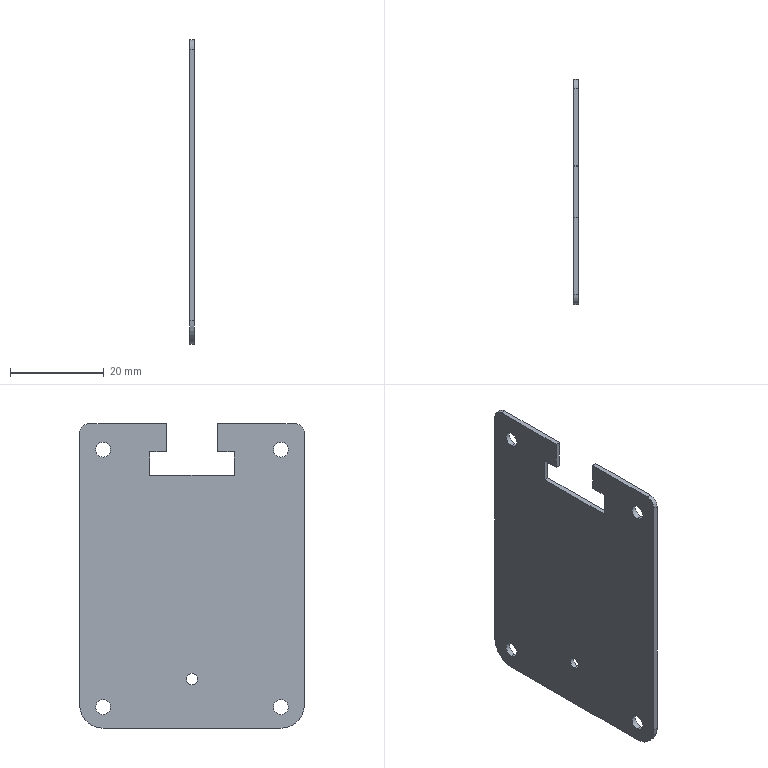Part | SolidWorks | features ICE 8, Fillet 2, Chamfer 1, Extrusion 1, HoleWzd 1 | 1 solid | 28 faces | box 1 x 48 x 65 mm | volume 2915 mm3 | cylinder 14 | plane 14 | commonest cylinder face diameters 3.2 x8 2.4 x2 4 x2 10 x2
STEP:
#1=CARTESIAN_POINT('',(20.,-19.,-26.4));
#2=VERTEX_POINT('',#1);
#3=CARTESIAN_POINT('',(20.,-19.,-29.6));
#4=VERTEX_POINT('',#3);
#5=CARTESIAN_POINT('',(20.,-19.,-28.));
#6=DIRECTION('',(1.,0.,0.));
#7=DIRECTION('',(0.,0.,-1.));
#8=AXIS2_PLACEMENT_3D('',#5,#6,#7);
#9=CIRCLE('',#8,1.6);
#10=EDGE_CURVE('',#2,#4,#9,.T.);
#11=ORIENTED_EDGE('',*,*,#10,.T.);
#12=CARTESIAN_POINT('',(19.,-19.,-29.6));
#13=VERTEX_POINT('',#12);
#14=CARTESIAN_POINT('',(139.,-19.,-29.6));
#15=DIRECTION('',(-1.,0.,0.));
#16=VECTOR('',#15,1000.);
#17=LINE('',#14,#16);
#18=EDGE_CURVE('',#4,#13,#17,.T.);
#19=ORIENTED_EDGE('',*,*,#18,.T.);
#20=CARTESIAN_POINT('',(19.,-19.,-26.4));
#21=VERTEX_POINT('',#20);
#22=CARTESIAN_POINT('',(19.,-19.,-28.));
#23=DIRECTION('',(-1.,0.,0.));
#24=DIRECTION('',(0.,0.,1.));
#25=AXIS2_PLACEMENT_3D('',#22,#23,#24);
#26=CIRCLE('',#25,1.6);
#27=EDGE_CURVE('',#13,#21,#26,.T.);
#28=ORIENTED_EDGE('',*,*,#27,.T.);
#29=CARTESIAN_POINT('',(139.,-19.,-26.4));
#30=DIRECTION('',(-1.,0.,0.));
#31=VECTOR('',#30,1000.);
#32=LINE('',#29,#31);
#33=EDGE_CURVE('',#2,#21,#32,.T.);
#34=ORIENTED_EDGE('',*,*,#33,.F.);
#35=EDGE_LOOP('',(#11,#19,#28,#34));
#36=FACE_OUTER_BOUND('',#35,.T.);
#37=CARTESIAN_POINT('',(139.,-19.,-28.));
#38=DIRECTION('',(-1.,0.,0.));
#39=DIRECTION('',(0.,0.,1.));
#40=AXIS2_PLACEMENT_3D('',#37,#38,#39);
#41=CYLINDRICAL_SURFACE('',#40,1.6);
#42=ADVANCED_FACE('',(#36),#41,.F.);
#43=CARTESIAN_POINT('',(20.,-19.,28.6));
#44=VERTEX_POINT('',#43);
#45=CARTESIAN_POINT('',(20.,-19.,25.4));
#46=VERTEX_POINT('',#45);
#47=CARTESIAN_POINT('',(20.,-19.,27.));
#48=DIRECTION('',(1.,0.,0.));
#49=DIRECTION('',(0.,0.,-1.));
#50=AXIS2_PLACEMENT_3D('',#47,#48,#49);
#51=CIRCLE('',#50,1.6);
#52=EDGE_CURVE('',#44,#46,#51,.T.);
#53=ORIENTED_EDGE('',*,*,#52,.T.);
#54=CARTESIAN_POINT('',(19.,-19.,25.4));
#55=VERTEX_POINT('',#54);
#56=CARTESIAN_POINT('',(139.,-19.,25.4));
#57=DIRECTION('',(-1.,0.,0.));
#58=VECTOR('',#57,1000.);
#59=LINE('',#56,#58);
#60=EDGE_CURVE('',#46,#55,#59,.T.);
#61=ORIENTED_EDGE('',*,*,#60,.T.);
#62=CARTESIAN_POINT('',(19.,-19.,28.6));
#63=VERTEX_POINT('',#62);
#64=CARTESIAN_POINT('',(19.,-19.,27.));
#65=DIRECTION('',(-1.,0.,0.));
#66=DIRECTION('',(0.,0.,1.));
#67=AXIS2_PLACEMENT_3D('',#64,#65,#66);
#68=CIRCLE('',#67,1.6);
#69=EDGE_CURVE('',#55,#63,#68,.T.);
#70=ORIENTED_EDGE('',*,*,#69,.T.);
#71=CARTESIAN_POINT('',(139.,-19.,28.6));
#72=DIRECTION('',(-1.,0.,0.));
#73=VECTOR('',#72,1000.);
#74=LINE('',#71,#73);
#75=EDGE_CURVE('',#44,#63,#74,.T.);
#76=ORIENTED_EDGE('',*,*,#75,.F.);
#77=EDGE_LOOP('',(#53,#61,#70,#76));
#78=FACE_OUTER_BOUND('',#77,.T.);
#79=CARTESIAN_POINT('',(139.,-19.,27.));
#80=DIRECTION('',(-1.,0.,0.));
#81=DIRECTION('',(0.,0.,1.));
#82=AXIS2_PLACEMENT_3D('',#79,#80,#81);
#83=CYLINDRICAL_SURFACE('',#82,1.6);
#84=ADVANCED_FACE('',(#78),#83,.F.);
#85=CARTESIAN_POINT('',(20.,19.,28.6));
#86=VERTEX_POINT('',#85);
#87=CARTESIAN_POINT('',(20.,19.,25.4));
#88=VERTEX_POINT('',#87);
#89=CARTESIAN_POINT('',(20.,19.,27.));
#90=DIRECTION('',(1.,0.,0.));
#91=DIRECTION('',(0.,0.,-1.));
#92=AXIS2_PLACEMENT_3D('',#89,#90,#91);
#93=CIRCLE('',#92,1.6);
#94=EDGE_CURVE('',#86,#88,#93,.T.);
#95=ORIENTED_EDGE('',*,*,#94,.T.);
#96=CARTESIAN_POINT('',(19.,19.,25.4));
#97=VERTEX_POINT('',#96);
#98=CARTESIAN_POINT('',(139.,19.,25.4));
#99=DIRECTION('',(-1.,0.,0.));
#100=VECTOR('',#99,1000.);
#101=LINE('',#98,#100);
#102=EDGE_CURVE('',#88,#97,#101,.T.);
#103=ORIENTED_EDGE('',*,*,#102,.T.);
#104=CARTESIAN_POINT('',(19.,19.,28.6));
#105=VERTEX_POINT('',#104);
#106=CARTESIAN_POINT('',(19.,19.,27.));
#107=DIRECTION('',(-1.,0.,0.));
#108=DIRECTION('',(0.,0.,-1.));
#109=AXIS2_PLACEMENT_3D('',#106,#107,#108);
#110=CIRCLE('',#109,1.6);
#111=EDGE_CURVE('',#97,#105,#110,.T.);
#112=ORIENTED_EDGE('',*,*,#111,.T.);
#113=CARTESIAN_POINT('',(139.,19.,28.6));
#114=DIRECTION('',(-1.,0.,0.));
#115=VECTOR('',#114,1000.);
#116=LINE('',#113,#115);
#117=EDGE_CURVE('',#86,#105,#116,.T.);
#118=ORIENTED_EDGE('',*,*,#117,.F.);
#119=EDGE_LOOP('',(#95,#103,#112,#118));
#120=FACE_OUTER_BOUND('',#119,.T.);
#121=CARTESIAN_POINT('',(139.,19.,27.));
#122=DIRECTION('',(-1.,0.,0.));
#123=DIRECTION('',(0.,0.,1.));
#124=AXIS2_PLACEMENT_3D('',#121,#122,#123);
#125=CYLINDRICAL_SURFACE('',#124,1.6);
#126=ADVANCED_FACE('',(#120),#125,.F.);
#127=CARTESIAN_POINT('',(20.,19.,-26.4));
#128=VERTEX_POINT('',#127);
#129=CARTESIAN_POINT('',(20.,19.,-29.6));
#130=VERTEX_POINT('',#129);
#131=CARTESIAN_POINT('',(20.,19.,-28.));
#132=DIRECTION('',(1.,0.,0.));
#133=DIRECTION('',(0.,0.,-1.));
#134=AXIS2_PLACEMENT_3D('',#131,#132,#133);
#135=CIRCLE('',#134,1.6);
#136=EDGE_CURVE('',#128,#130,#135,.T.);
#137=ORIENTED_EDGE('',*,*,#136,.T.);
#138=CARTESIAN_POINT('',(19.,19.,-29.6));
#139=VERTEX_POINT('',#138);
#140=CARTESIAN_POINT('',(139.,19.,-29.6));
#141=DIRECTION('',(-1.,0.,0.));
#142=VECTOR('',#141,1000.);
#143=LINE('',#140,#142);
#144=EDGE_CURVE('',#130,#139,#143,.T.);
#145=ORIENTED_EDGE('',*,*,#144,.T.);
#146=CARTESIAN_POINT('',(19.,19.,-26.4));
#147=VERTEX_POINT('',#146);
#148=CARTESIAN_POINT('',(19.,19.,-28.));
#149=DIRECTION('',(-1.,0.,0.));
#150=DIRECTION('',(0.,0.,1.));
#151=AXIS2_PLACEMENT_3D('',#148,#149,#150);
#152=CIRCLE('',#151,1.6);
#153=EDGE_CURVE('',#139,#147,#152,.T.);
#154=ORIENTED_EDGE('',*,*,#153,.T.);
#155=CARTESIAN_POINT('',(139.,19.,-26.4));
#156=DIRECTION('',(-1.,0.,0.));
#157=VECTOR('',#156,1000.);
#158=LINE('',#155,#157);
#159=EDGE_CURVE('',#128,#147,#158,.T.);
#160=ORIENTED_EDGE('',*,*,#159,.F.);
#161=EDGE_LOOP('',(#137,#145,#154,#160));
#162=FACE_OUTER_BOUND('',#161,.T.);
#163=CARTESIAN_POINT('',(139.,19.,-28.));
#164=DIRECTION('',(-1.,0.,0.));
#165=DIRECTION('',(0.,0.,1.));
#166=AXIS2_PLACEMENT_3D('',#163,#164,#165);
#167=CYLINDRICAL_SURFACE('',#166,1.6);
#168=ADVANCED_FACE('',(#162),#167,.F.);
#169=CARTESIAN_POINT('',(19.,0.,-23.2));
#170=VERTEX_POINT('',#169);
#171=CARTESIAN_POINT('',(19.,0.,-20.8));
#172=VERTEX_POINT('',#171);
#173=CARTESIAN_POINT('',(19.,0.,-22.));
#174=DIRECTION('',(-1.,0.,0.));
#175=DIRECTION('',(0.,0.,-1.));
#176=AXIS2_PLACEMENT_3D('',#173,#174,#175);
#177=CIRCLE('',#176,1.2);
#178=EDGE_CURVE('',#170,#172,#177,.T.);
#179=ORIENTED_EDGE('',*,*,#178,.T.);
#180=CARTESIAN_POINT('',(20.,0.,-20.8));
#181=VERTEX_POINT('',#180);
#182=CARTESIAN_POINT('',(14.,0.,-20.8));
#183=DIRECTION('',(1.,0.,0.));
#184=VECTOR('',#183,1000.);
#185=LINE('',#182,#184);
#186=EDGE_CURVE('',#172,#181,#185,.T.);
#187=ORIENTED_EDGE('',*,*,#186,.T.);
#188=CARTESIAN_POINT('',(20.,0.,-23.2));
#189=VERTEX_POINT('',#188);
#190=CARTESIAN_POINT('',(20.,0.,-22.));
#191=DIRECTION('',(1.,0.,0.));
#192=DIRECTION('',(0.,0.,-1.));
#193=AXIS2_PLACEMENT_3D('',#190,#191,#192);
#194=CIRCLE('',#193,1.2);
#195=EDGE_CURVE('',#181,#189,#194,.T.);
#196=ORIENTED_EDGE('',*,*,#195,.T.);
#197=CARTESIAN_POINT('',(14.,0.,-23.2));
#198=DIRECTION('',(1.,0.,0.));
#199=VECTOR('',#198,1000.);
#200=LINE('',#197,#199);
#201=EDGE_CURVE('',#170,#189,#200,.T.);
#202=ORIENTED_EDGE('',*,*,#201,.F.);
#203=EDGE_LOOP('',(#179,#187,#196,#202));
#204=FACE_OUTER_BOUND('',#203,.T.);
#205=CARTESIAN_POINT('',(14.,0.,-22.));
#206=DIRECTION('',(1.,0.,0.));
#207=DIRECTION('',(0.,0.,-1.));
#208=AXIS2_PLACEMENT_3D('',#205,#206,#207);
#209=CYLINDRICAL_SURFACE('',#208,1.2);
#210=ADVANCED_FACE('',(#204),#209,.F.);
#211=CARTESIAN_POINT('',(20.,22.,32.5));
#212=VERTEX_POINT('',#211);
#213=CARTESIAN_POINT('',(20.,5.5,32.5));
#214=VERTEX_POINT('',#213);
#215=CARTESIAN_POINT('',(20.,24.,32.5));
#216=DIRECTION('',(0.,-1.,0.));
#217=VECTOR('',#216,1000.);
#218=LINE('',#215,#217);
#219=EDGE_CURVE('',#212,#214,#218,.T.);
#220=ORIENTED_EDGE('',*,*,#219,.F.);
#221=CARTESIAN_POINT('',(19.,22.,32.5));
#222=VERTEX_POINT('',#221);
#223=CARTESIAN_POINT('',(20.,22.,32.5));
#224=DIRECTION('',(-1.,0.,0.));
#225=VECTOR('',#224,1000.);
#226=LINE('',#223,#225);
#227=EDGE_CURVE('',#212,#222,#226,.T.);
#228=ORIENTED_EDGE('',*,*,#227,.T.);
#229=CARTESIAN_POINT('',(19.,5.5,32.5));
#230=VERTEX_POINT('',#229);
#231=CARTESIAN_POINT('',(19.,24.,32.5));
#232=DIRECTION('',(0.,-1.,0.));
#233=VECTOR('',#232,1000.);
#234=LINE('',#231,#233);
#235=EDGE_CURVE('',#222,#230,#234,.T.);
#236=ORIENTED_EDGE('',*,*,#235,.T.);
#237=CARTESIAN_POINT('',(-60.,5.5,32.5));
#238=DIRECTION('',(1.,0.,0.));
#239=VECTOR('',#238,1000.);
#240=LINE('',#237,#239);
#241=EDGE_CURVE('',#230,#214,#240,.T.);
#242=ORIENTED_EDGE('',*,*,#241,.T.);
#243=EDGE_LOOP('',(#220,#228,#236,#242));
#244=FACE_OUTER_BOUND('',#243,.T.);
#245=CARTESIAN_POINT('',(20.,24.,32.5));
#246=DIRECTION('',(0.,0.,-1.));
#247=DIRECTION('',(0.,1.,0.));
#248=AXIS2_PLACEMENT_3D('',#245,#246,#247);
#249=PLANE('',#248);
#250=ADVANCED_FACE('',(#244),#249,.F.);
#251=CARTESIAN_POINT('',(20.,-19.,-32.5));
#252=VERTEX_POINT('',#251);
#253=CARTESIAN_POINT('',(19.,-19.,-32.5));
#254=VERTEX_POINT('',#253);
#255=CARTESIAN_POINT('',(20.,-19.,-32.5));
#256=DIRECTION('',(-1.,0.,0.));
#257=VECTOR('',#256,1000.);
#258=LINE('',#255,#257);
#259=EDGE_CURVE('',#252,#254,#258,.T.);
#260=ORIENTED_EDGE('',*,*,#259,.T.);
#261=CARTESIAN_POINT('',(19.,19.,-32.5));
#262=VERTEX_POINT('',#261);
#263=CARTESIAN_POINT('',(19.,24.,-32.5));
#264=DIRECTION('',(0.,1.,0.));
#265=VECTOR('',#264,1000.);
#266=LINE('',#263,#265);
#267=EDGE_CURVE('',#254,#262,#266,.T.);
#268=ORIENTED_EDGE('',*,*,#267,.T.);
#269=CARTESIAN_POINT('',(20.,19.,-32.5));
#270=VERTEX_POINT('',#269);
#271=CARTESIAN_POINT('',(20.,19.,-32.5));
#272=DIRECTION('',(1.,0.,0.));
#273=VECTOR('',#272,1000.);
#274=LINE('',#271,#273);
#275=EDGE_CURVE('',#262,#270,#274,.T.);
#276=ORIENTED_EDGE('',*,*,#275,.T.);
#277=CARTESIAN_POINT('',(20.,24.,-32.5));
#278=DIRECTION('',(0.,1.,0.));
#279=VECTOR('',#278,1000.);
#280=LINE('',#277,#279);
#281=EDGE_CURVE('',#252,#270,#280,.T.);
#282=ORIENTED_EDGE('',*,*,#281,.F.);
#283=EDGE_LOOP('',(#260,#268,#276,#282));
#284=FACE_OUTER_BOUND('',#283,.T.);
#285=CARTESIAN_POINT('',(20.,24.,-32.5));
#286=DIRECTION('',(0.,0.,1.));
#287=DIRECTION('',(0.,-1.,0.));
#288=AXIS2_PLACEMENT_3D('',#285,#286,#287);
#289=PLANE('',#288);
#290=ADVANCED_FACE('',(#284),#289,.F.);
#291=CARTESIAN_POINT('',(19.,24.,30.5));
#292=VERTEX_POINT('',#291);
#293=CARTESIAN_POINT('',(19.,24.,-27.5));
#294=VERTEX_POINT('',#293);
#295=CARTESIAN_POINT('',(19.,24.,-41.997));
#296=DIRECTION('',(0.,0.,-1.));
#297=VECTOR('',#296,1000.);
#298=LINE('',#295,#297);
#299=EDGE_CURVE('',#292,#294,#298,.T.);
#300=ORIENTED_EDGE('',*,*,#299,.F.);
#301=CARTESIAN_POINT('',(20.,24.,30.5));
#302=VERTEX_POINT('',#301);
#303=CARTESIAN_POINT('',(20.,24.,30.5));
#304=DIRECTION('',(1.,0.,0.));
#305=VECTOR('',#304,1000.);
#306=LINE('',#303,#305);
#307=EDGE_CURVE('',#292,#302,#306,.T.);
#308=ORIENTED_EDGE('',*,*,#307,.T.);
#309=CARTESIAN_POINT('',(20.,24.,-27.5));
#310=VERTEX_POINT('',#309);
#311=CARTESIAN_POINT('',(20.,24.,32.5));
#312=DIRECTION('',(0.,0.,1.));
#313=VECTOR('',#312,1000.);
#314=LINE('',#311,#313);
#315=EDGE_CURVE('',#310,#302,#314,.T.);
#316=ORIENTED_EDGE('',*,*,#315,.F.);
#317=CARTESIAN_POINT('',(20.,24.,-27.5));
#318=DIRECTION('',(-1.,0.,0.));
#319=VECTOR('',#318,1000.);
#320=LINE('',#317,#319);
#321=EDGE_CURVE('',#310,#294,#320,.T.);
#322=ORIENTED_EDGE('',*,*,#321,.T.);
#323=EDGE_LOOP('',(#300,#308,#316,#322));
#324=FACE_OUTER_BOUND('',#323,.T.);
#325=CARTESIAN_POINT('',(20.,24.,32.5));
#326=DIRECTION('',(0.,-1.,0.));
#327=DIRECTION('',(0.,0.,-1.));
#328=AXIS2_PLACEMENT_3D('',#325,#326,#327);
#329=PLANE('',#328);
#330=ADVANCED_FACE('',(#324),#329,.F.);
#331=CARTESIAN_POINT('',(19.,-5.5,32.5));
#332=VERTEX_POINT('',#331);
#333=CARTESIAN_POINT('',(19.,-22.,32.5));
#334=VERTEX_POINT('',#333);
#335=CARTESIAN_POINT('',(19.,24.,32.5));
#336=DIRECTION('',(0.,-1.,0.));
#337=VECTOR('',#336,1000.);
#338=LINE('',#335,#337);
#339=EDGE_CURVE('',#332,#334,#338,.T.);
#340=ORIENTED_EDGE('',*,*,#339,.T.);
#341=CARTESIAN_POINT('',(20.,-22.,32.5));
#342=VERTEX_POINT('',#341);
#343=CARTESIAN_POINT('',(20.,-22.,32.5));
#344=DIRECTION('',(1.,0.,0.));
#345=VECTOR('',#344,1000.);
#346=LINE('',#343,#345);
#347=EDGE_CURVE('',#334,#342,#346,.T.);
#348=ORIENTED_EDGE('',*,*,#347,.T.);
#349=CARTESIAN_POINT('',(20.,-5.5,32.5));
#350=VERTEX_POINT('',#349);
#351=CARTESIAN_POINT('',(20.,24.,32.5));
#352=DIRECTION('',(0.,-1.,0.));
#353=VECTOR('',#352,1000.);
#354=LINE('',#351,#353);
#355=EDGE_CURVE('',#350,#342,#354,.T.);
#356=ORIENTED_EDGE('',*,*,#355,.F.);
#357=CARTESIAN_POINT('',(-60.,-5.5,32.5));
#358=DIRECTION('',(1.,0.,0.));
#359=VECTOR('',#358,1000.);
#360=LINE('',#357,#359);
#361=EDGE_CURVE('',#332,#350,#360,.T.);
#362=ORIENTED_EDGE('',*,*,#361,.F.);
#363=EDGE_LOOP('',(#340,#348,#356,#362));
#364=FACE_OUTER_BOUND('',#363,.T.);
#365=CARTESIAN_POINT('',(20.,24.,32.5));
#366=DIRECTION('',(0.,0.,-1.));
#367=DIRECTION('',(0.,1.,0.));
#368=AXIS2_PLACEMENT_3D('',#365,#366,#367);
#369=PLANE('',#368);
#370=ADVANCED_FACE('',(#364),#369,.F.);
#371=CARTESIAN_POINT('',(20.,-24.,30.5));
#372=VERTEX_POINT('',#371);
#373=CARTESIAN_POINT('',(20.,-24.,-27.5));
#374=VERTEX_POINT('',#373);
#375=CARTESIAN_POINT('',(20.,-24.,32.5));
#376=DIRECTION('',(0.,0.,-1.));
#377=VECTOR('',#376,1000.);
#378=LINE('',#375,#377);
#379=EDGE_CURVE('',#372,#374,#378,.T.);
#380=ORIENTED_EDGE('',*,*,#379,.F.);
#381=CARTESIAN_POINT('',(19.,-24.,30.5));
#382=VERTEX_POINT('',#381);
#383=CARTESIAN_POINT('',(20.,-24.,30.5));
#384=DIRECTION('',(-1.,0.,0.));
#385=VECTOR('',#384,1000.);
#386=LINE('',#383,#385);
#387=EDGE_CURVE('',#372,#382,#386,.T.);
#388=ORIENTED_EDGE('',*,*,#387,.T.);
#389=CARTESIAN_POINT('',(19.,-24.,-27.5));
#390=VERTEX_POINT('',#389);
#391=CARTESIAN_POINT('',(19.,-24.,32.5));
#392=DIRECTION('',(0.,0.,-1.));
#393=VECTOR('',#392,1000.);
#394=LINE('',#391,#393);
#395=EDGE_CURVE('',#382,#390,#394,.T.);
#396=ORIENTED_EDGE('',*,*,#395,.T.);
#397=CARTESIAN_POINT('',(20.,-24.,-27.5));
#398=DIRECTION('',(1.,0.,0.));
#399=VECTOR('',#398,1000.);
#400=LINE('',#397,#399);
#401=EDGE_CURVE('',#390,#374,#400,.T.);
#402=ORIENTED_EDGE('',*,*,#401,.T.);
#403=EDGE_LOOP('',(#380,#388,#396,#402));
#404=FACE_OUTER_BOUND('',#403,.T.);
#405=CARTESIAN_POINT('',(20.,-24.,32.5));
#406=DIRECTION('',(0.,1.,0.));
#407=DIRECTION('',(0.,0.,1.));
#408=AXIS2_PLACEMENT_3D('',#405,#406,#407);
#409=PLANE('',#408);
#410=ADVANCED_FACE('',(#404),#409,.F.);
#411=ORIENTED_EDGE('',*,*,#10,.F.);
#412=CARTESIAN_POINT('',(20.,-19.,-28.));
#413=DIRECTION('',(1.,0.,0.));
#414=DIRECTION('',(0.,0.,-1.));
#415=AXIS2_PLACEMENT_3D('',#412,#413,#414);
#416=CIRCLE('',#415,1.6);
#417=EDGE_CURVE('',#4,#2,#416,.T.);
#418=ORIENTED_EDGE('',*,*,#417,.F.);
#419=EDGE_LOOP('',(#411,#418));
#420=FACE_BOUND('',#419,.T.);
#421=ORIENTED_EDGE('',*,*,#52,.F.);
#422=CARTESIAN_POINT('',(20.,-19.,27.));
#423=DIRECTION('',(1.,0.,0.));
#424=DIRECTION('',(0.,0.,-1.));
#425=AXIS2_PLACEMENT_3D('',#422,#423,#424);
#426=CIRCLE('',#425,1.6);
#427=EDGE_CURVE('',#46,#44,#426,.T.);
#428=ORIENTED_EDGE('',*,*,#427,.F.);
#429=EDGE_LOOP('',(#421,#428));
#430=FACE_BOUND('',#429,.T.);
#431=ORIENTED_EDGE('',*,*,#94,.F.);
#432=CARTESIAN_POINT('',(20.,19.,27.));
#433=DIRECTION('',(1.,0.,0.));
#434=DIRECTION('',(0.,0.,-1.));
#435=AXIS2_PLACEMENT_3D('',#432,#433,#434);
#436=CIRCLE('',#435,1.6);
#437=EDGE_CURVE('',#88,#86,#436,.T.);
#438=ORIENTED_EDGE('',*,*,#437,.F.);
#439=EDGE_LOOP('',(#431,#438));
#440=FACE_BOUND('',#439,.T.);
#441=ORIENTED_EDGE('',*,*,#136,.F.);
#442=CARTESIAN_POINT('',(20.,19.,-28.));
#443=DIRECTION('',(1.,0.,0.));
#444=DIRECTION('',(0.,0.,-1.));
#445=AXIS2_PLACEMENT_3D('',#442,#443,#444);
#446=CIRCLE('',#445,1.6);
#447=EDGE_CURVE('',#130,#128,#446,.T.);
#448=ORIENTED_EDGE('',*,*,#447,.F.);
#449=EDGE_LOOP('',(#441,#448));
#450=FACE_BOUND('',#449,.T.);
#451=CARTESIAN_POINT('',(20.,0.,-22.));
#452=DIRECTION('',(1.,0.,0.));
#453=DIRECTION('',(0.,0.,-1.));
#454=AXIS2_PLACEMENT_3D('',#451,#452,#453);
#455=CIRCLE('',#454,1.2);
#456=EDGE_CURVE('',#189,#181,#455,.T.);
#457=ORIENTED_EDGE('',*,*,#456,.F.);
#458=ORIENTED_EDGE('',*,*,#195,.F.);
#459=EDGE_LOOP('',(#457,#458));
#460=FACE_BOUND('',#459,.T.);
#461=ORIENTED_EDGE('',*,*,#315,.T.);
#462=CARTESIAN_POINT('',(20.,22.,30.5));
#463=DIRECTION('',(1.,0.,0.));
#464=DIRECTION('',(0.,0.,-1.));
#465=AXIS2_PLACEMENT_3D('',#462,#463,#464);
#466=CIRCLE('',#465,2.);
#467=EDGE_CURVE('',#302,#212,#466,.T.);
#468=ORIENTED_EDGE('',*,*,#467,.T.);
#469=ORIENTED_EDGE('',*,*,#219,.T.);
#470=CARTESIAN_POINT('',(20.,5.5,26.5));
#471=VERTEX_POINT('',#470);
#472=CARTESIAN_POINT('',(20.,5.5,32.5));
#473=DIRECTION('',(0.,0.,1.));
#474=VECTOR('',#473,1000.);
#475=LINE('',#472,#474);
#476=EDGE_CURVE('',#471,#214,#475,.T.);
#477=ORIENTED_EDGE('',*,*,#476,.F.);
#478=CARTESIAN_POINT('',(20.,9.,26.5));
#479=VERTEX_POINT('',#478);
#480=CARTESIAN_POINT('',(20.,5.5,26.5));
#481=DIRECTION('',(0.,-1.,0.));
#482=VECTOR('',#481,1000.);
#483=LINE('',#480,#482);
#484=EDGE_CURVE('',#479,#471,#483,.T.);
#485=ORIENTED_EDGE('',*,*,#484,.F.);
#486=CARTESIAN_POINT('',(20.,9.,21.5));
#487=VERTEX_POINT('',#486);
#488=CARTESIAN_POINT('',(20.,9.,26.5));
#489=DIRECTION('',(0.,0.,1.));
#490=VECTOR('',#489,1000.);
#491=LINE('',#488,#490);
#492=EDGE_CURVE('',#487,#479,#491,.T.);
#493=ORIENTED_EDGE('',*,*,#492,.F.);
#494=CARTESIAN_POINT('',(20.,-9.,21.5));
#495=VERTEX_POINT('',#494);
#496=CARTESIAN_POINT('',(20.,9.,21.5));
#497=DIRECTION('',(0.,1.,0.));
#498=VECTOR('',#497,1000.);
#499=LINE('',#496,#498);
#500=EDGE_CURVE('',#495,#487,#499,.T.);
#501=ORIENTED_EDGE('',*,*,#500,.F.);
#502=CARTESIAN_POINT('',(20.,-9.,26.5));
#503=VERTEX_POINT('',#502);
#504=CARTESIAN_POINT('',(20.,-9.,26.5));
#505=DIRECTION('',(0.,0.,-1.));
#506=VECTOR('',#505,1000.);
#507=LINE('',#504,#506);
#508=EDGE_CURVE('',#503,#495,#507,.T.);
#509=ORIENTED_EDGE('',*,*,#508,.F.);
#510=CARTESIAN_POINT('',(20.,-5.5,26.5));
#511=VERTEX_POINT('',#510);
#512=CARTESIAN_POINT('',(20.,-5.5,26.5));
#513=DIRECTION('',(0.,-1.,0.));
#514=VECTOR('',#513,1000.);
#515=LINE('',#512,#514);
#516=EDGE_CURVE('',#511,#503,#515,.T.);
#517=ORIENTED_EDGE('',*,*,#516,.F.);
#518=CARTESIAN_POINT('',(20.,-5.5,32.5));
#519=DIRECTION('',(0.,0.,-1.));
#520=VECTOR('',#519,1000.);
#521=LINE('',#518,#520);
#522=EDGE_CURVE('',#350,#511,#521,.T.);
#523=ORIENTED_EDGE('',*,*,#522,.F.);
#524=ORIENTED_EDGE('',*,*,#355,.T.);
#525=CARTESIAN_POINT('',(20.,-22.,30.5));
#526=DIRECTION('',(1.,0.,0.));
#527=DIRECTION('',(0.,0.,-1.));
#528=AXIS2_PLACEMENT_3D('',#525,#526,#527);
#529=CIRCLE('',#528,2.);
#530=EDGE_CURVE('',#342,#372,#529,.T.);
#531=ORIENTED_EDGE('',*,*,#530,.T.);
#532=ORIENTED_EDGE('',*,*,#379,.T.);
#533=CARTESIAN_POINT('',(20.,-19.,-27.5));
#534=DIRECTION('',(1.,0.,0.));
#535=DIRECTION('',(0.,0.,-1.));
#536=AXIS2_PLACEMENT_3D('',#533,#534,#535);
#537=CIRCLE('',#536,5.);
#538=EDGE_CURVE('',#374,#252,#537,.T.);
#539=ORIENTED_EDGE('',*,*,#538,.T.);
#540=ORIENTED_EDGE('',*,*,#281,.T.);
#541=CARTESIAN_POINT('',(20.,19.,-27.5));
#542=DIRECTION('',(1.,0.,0.));
#543=DIRECTION('',(0.,0.,-1.));
#544=AXIS2_PLACEMENT_3D('',#541,#542,#543);
#545=CIRCLE('',#544,5.);
#546=EDGE_CURVE('',#270,#310,#545,.T.);
#547=ORIENTED_EDGE('',*,*,#546,.T.);
#548=EDGE_LOOP('',(#461,#468,#469,#477,#485,#493,#501,#509,#517,#523,#524,#531,#532,#539,#540,#547));
#549=FACE_OUTER_BOUND('',#548,.T.);
#550=CARTESIAN_POINT('',(20.,0.,0.));
#551=DIRECTION('',(1.,0.,0.));
#552=DIRECTION('',(0.,0.,-1.));
#553=AXIS2_PLACEMENT_3D('',#550,#551,#552);
#554=PLANE('',#553);
#555=ADVANCED_FACE('',(#420,#430,#440,#450,#460,#549),#554,.T.);
#556=ORIENTED_EDGE('',*,*,#241,.F.);
#557=CARTESIAN_POINT('',(19.,5.5,26.5));
#558=VERTEX_POINT('',#557);
#559=CARTESIAN_POINT('',(19.,5.5,32.5));
#560=DIRECTION('',(0.,0.,-1.));
#561=VECTOR('',#560,1000.);
#562=LINE('',#559,#561);
#563=EDGE_CURVE('',#230,#558,#562,.T.);
#564=ORIENTED_EDGE('',*,*,#563,.T.);
#565=CARTESIAN_POINT('',(-60.,5.5,26.5));
#566=DIRECTION('',(1.,0.,0.));
#567=VECTOR('',#566,1000.);
#568=LINE('',#565,#567);
#569=EDGE_CURVE('',#558,#471,#568,.T.);
#570=ORIENTED_EDGE('',*,*,#569,.T.);
#571=ORIENTED_EDGE('',*,*,#476,.T.);
#572=EDGE_LOOP('',(#556,#564,#570,#571));
#573=FACE_OUTER_BOUND('',#572,.T.);
#574=CARTESIAN_POINT('',(-60.,5.5,32.5));
#575=DIRECTION('',(0.,1.,0.));
#576=DIRECTION('',(0.,0.,1.));
#577=AXIS2_PLACEMENT_3D('',#574,#575,#576);
#578=PLANE('',#577);
#579=ADVANCED_FACE('',(#573),#578,.F.);
#580=ORIENTED_EDGE('',*,*,#569,.F.);
#581=CARTESIAN_POINT('',(19.,9.,26.5));
#582=VERTEX_POINT('',#581);
#583=CARTESIAN_POINT('',(19.,5.5,26.5));
#584=DIRECTION('',(0.,1.,0.));
#585=VECTOR('',#584,1000.);
#586=LINE('',#583,#585);
#587=EDGE_CURVE('',#558,#582,#586,.T.);
#588=ORIENTED_EDGE('',*,*,#587,.T.);
#589=CARTESIAN_POINT('',(-60.,9.,26.5));
#590=DIRECTION('',(1.,0.,0.));
#591=VECTOR('',#590,1000.);
#592=LINE('',#589,#591);
#593=EDGE_CURVE('',#582,#479,#592,.T.);
#594=ORIENTED_EDGE('',*,*,#593,.T.);
#595=ORIENTED_EDGE('',*,*,#484,.T.);
#596=EDGE_LOOP('',(#580,#588,#594,#595));
#597=FACE_OUTER_BOUND('',#596,.T.);
#598=CARTESIAN_POINT('',(-60.,5.5,26.5));
#599=DIRECTION('',(0.,0.,1.));
#600=DIRECTION('',(1.,0.,0.));
#601=AXIS2_PLACEMENT_3D('',#598,#599,#600);
#602=PLANE('',#601);
#603=ADVANCED_FACE('',(#597),#602,.F.);
#604=ORIENTED_EDGE('',*,*,#593,.F.);
#605=CARTESIAN_POINT('',(19.,9.,21.5));
#606=VERTEX_POINT('',#605);
#607=CARTESIAN_POINT('',(19.,9.,26.5));
#608=DIRECTION('',(0.,0.,-1.));
#609=VECTOR('',#608,1000.);
#610=LINE('',#607,#609);
#611=EDGE_CURVE('',#582,#606,#610,.T.);
#612=ORIENTED_EDGE('',*,*,#611,.T.);
#613=CARTESIAN_POINT('',(-60.,9.,21.5));
#614=DIRECTION('',(1.,0.,0.));
#615=VECTOR('',#614,1000.);
#616=LINE('',#613,#615);
#617=EDGE_CURVE('',#606,#487,#616,.T.);
#618=ORIENTED_EDGE('',*,*,#617,.T.);
#619=ORIENTED_EDGE('',*,*,#492,.T.);
#620=EDGE_LOOP('',(#604,#612,#618,#619));
#621=FACE_OUTER_BOUND('',#620,.T.);
#622=CARTESIAN_POINT('',(-60.,9.,26.5));
#623=DIRECTION('',(0.,1.,0.));
#624=DIRECTION('',(0.,0.,1.));
#625=AXIS2_PLACEMENT_3D('',#622,#623,#624);
#626=PLANE('',#625);
#627=ADVANCED_FACE('',(#621),#626,.F.);
#628=ORIENTED_EDGE('',*,*,#617,.F.);
#629=CARTESIAN_POINT('',(19.,-9.,21.5));
#630=VERTEX_POINT('',#629);
#631=CARTESIAN_POINT('',(19.,9.,21.5));
#632=DIRECTION('',(0.,-1.,0.));
#633=VECTOR('',#632,1000.);
#634=LINE('',#631,#633);
#635=EDGE_CURVE('',#606,#630,#634,.T.);
#636=ORIENTED_EDGE('',*,*,#635,.T.);
#637=CARTESIAN_POINT('',(-60.,-9.,21.5));
#638=DIRECTION('',(1.,0.,0.));
#639=VECTOR('',#638,1000.);
#640=LINE('',#637,#639);
#641=EDGE_CURVE('',#630,#495,#640,.T.);
#642=ORIENTED_EDGE('',*,*,#641,.T.);
#643=ORIENTED_EDGE('',*,*,#500,.T.);
#644=EDGE_LOOP('',(#628,#636,#642,#643));
#645=FACE_OUTER_BOUND('',#644,.T.);
#646=CARTESIAN_POINT('',(-60.,9.,21.5));
#647=DIRECTION('',(0.,0.,-1.));
#648=DIRECTION('',(0.,1.,0.));
#649=AXIS2_PLACEMENT_3D('',#646,#647,#648);
#650=PLANE('',#649);
#651=ADVANCED_FACE('',(#645),#650,.F.);
#652=ORIENTED_EDGE('',*,*,#641,.F.);
#653=CARTESIAN_POINT('',(19.,-9.,26.5));
#654=VERTEX_POINT('',#653);
#655=CARTESIAN_POINT('',(19.,-9.,26.5));
#656=DIRECTION('',(0.,0.,1.));
#657=VECTOR('',#656,1000.);
#658=LINE('',#655,#657);
#659=EDGE_CURVE('',#630,#654,#658,.T.);
#660=ORIENTED_EDGE('',*,*,#659,.T.);
#661=CARTESIAN_POINT('',(-60.,-9.,26.5));
#662=DIRECTION('',(1.,0.,0.));
#663=VECTOR('',#662,1000.);
#664=LINE('',#661,#663);
#665=EDGE_CURVE('',#654,#503,#664,.T.);
#666=ORIENTED_EDGE('',*,*,#665,.T.);
#667=ORIENTED_EDGE('',*,*,#508,.T.);
#668=EDGE_LOOP('',(#652,#660,#666,#667));
#669=FACE_OUTER_BOUND('',#668,.T.);
#670=CARTESIAN_POINT('',(-60.,-9.,26.5));
#671=DIRECTION('',(0.,-1.,0.));
#672=DIRECTION('',(0.,0.,-1.));
#673=AXIS2_PLACEMENT_3D('',#670,#671,#672);
#674=PLANE('',#673);
#675=ADVANCED_FACE('',(#669),#674,.F.);
#676=ORIENTED_EDGE('',*,*,#665,.F.);
#677=CARTESIAN_POINT('',(19.,-5.5,26.5));
#678=VERTEX_POINT('',#677);
#679=CARTESIAN_POINT('',(19.,-5.5,26.5));
#680=DIRECTION('',(0.,1.,0.));
#681=VECTOR('',#680,1000.);
#682=LINE('',#679,#681);
#683=EDGE_CURVE('',#654,#678,#682,.T.);
#684=ORIENTED_EDGE('',*,*,#683,.T.);
#685=CARTESIAN_POINT('',(-60.,-5.5,26.5));
#686=DIRECTION('',(1.,0.,0.));
#687=VECTOR('',#686,1000.);
#688=LINE('',#685,#687);
#689=EDGE_CURVE('',#678,#511,#688,.T.);
#690=ORIENTED_EDGE('',*,*,#689,.T.);
#691=ORIENTED_EDGE('',*,*,#516,.T.);
#692=EDGE_LOOP('',(#676,#684,#690,#691));
#693=FACE_OUTER_BOUND('',#692,.T.);
#694=CARTESIAN_POINT('',(-60.,-5.5,26.5));
#695=DIRECTION('',(0.,0.,1.));
#696=DIRECTION('',(0.,-1.,0.));
#697=AXIS2_PLACEMENT_3D('',#694,#695,#696);
#698=PLANE('',#697);
#699=ADVANCED_FACE('',(#693),#698,.F.);
#700=ORIENTED_EDGE('',*,*,#689,.F.);
#701=CARTESIAN_POINT('',(19.,-5.5,32.5));
#702=DIRECTION('',(0.,0.,1.));
#703=VECTOR('',#702,1000.);
#704=LINE('',#701,#703);
#705=EDGE_CURVE('',#678,#332,#704,.T.);
#706=ORIENTED_EDGE('',*,*,#705,.T.);
#707=ORIENTED_EDGE('',*,*,#361,.T.);
#708=ORIENTED_EDGE('',*,*,#522,.T.);
#709=EDGE_LOOP('',(#700,#706,#707,#708));
#710=FACE_OUTER_BOUND('',#709,.T.);
#711=CARTESIAN_POINT('',(-60.,-5.5,32.5));
#712=DIRECTION('',(0.,-1.,0.));
#713=DIRECTION('',(0.,0.,-1.));
#714=AXIS2_PLACEMENT_3D('',#711,#712,#713);
#715=PLANE('',#714);
#716=ADVANCED_FACE('',(#710),#715,.F.);
#717=ORIENTED_EDGE('',*,*,#186,.F.);
#718=CARTESIAN_POINT('',(19.,0.,-22.));
#719=DIRECTION('',(-1.,0.,0.));
#720=DIRECTION('',(0.,0.,-1.));
#721=AXIS2_PLACEMENT_3D('',#718,#719,#720);
#722=CIRCLE('',#721,1.2);
#723=EDGE_CURVE('',#172,#170,#722,.T.);
#724=ORIENTED_EDGE('',*,*,#723,.T.);
#725=ORIENTED_EDGE('',*,*,#201,.T.);
#726=ORIENTED_EDGE('',*,*,#456,.T.);
#727=EDGE_LOOP('',(#717,#724,#725,#726));
#728=FACE_OUTER_BOUND('',#727,.T.);
#729=CARTESIAN_POINT('',(14.,0.,-22.));
#730=DIRECTION('',(1.,0.,0.));
#731=DIRECTION('',(0.,0.,-1.));
#732=AXIS2_PLACEMENT_3D('',#729,#730,#731);
#733=CYLINDRICAL_SURFACE('',#732,1.2);
#734=ADVANCED_FACE('',(#728),#733,.F.);
#735=CARTESIAN_POINT('',(19.,-19.,-27.5));
#736=DIRECTION('',(-1.,0.,0.));
#737=DIRECTION('',(0.,0.,-1.));
#738=AXIS2_PLACEMENT_3D('',#735,#736,#737);
#739=CIRCLE('',#738,5.);
#740=EDGE_CURVE('',#254,#390,#739,.T.);
#741=ORIENTED_EDGE('',*,*,#740,.F.);
#742=ORIENTED_EDGE('',*,*,#259,.F.);
#743=ORIENTED_EDGE('',*,*,#538,.F.);
#744=ORIENTED_EDGE('',*,*,#401,.F.);
#745=EDGE_LOOP('',(#741,#742,#743,#744));
#746=FACE_OUTER_BOUND('',#745,.T.);
#747=CARTESIAN_POINT('',(20.,-19.,-27.5));
#748=DIRECTION('',(-1.,0.,0.));
#749=DIRECTION('',(0.,0.,1.));
#750=AXIS2_PLACEMENT_3D('',#747,#748,#749);
#751=CYLINDRICAL_SURFACE('',#750,5.);
#752=ADVANCED_FACE('',(#746),#751,.T.);
#753=CARTESIAN_POINT('',(19.,19.,-27.5));
#754=DIRECTION('',(-1.,0.,0.));
#755=DIRECTION('',(0.,0.,-1.));
#756=AXIS2_PLACEMENT_3D('',#753,#754,#755);
#757=CIRCLE('',#756,5.);
#758=EDGE_CURVE('',#294,#262,#757,.T.);
#759=ORIENTED_EDGE('',*,*,#758,.F.);
#760=ORIENTED_EDGE('',*,*,#321,.F.);
#761=ORIENTED_EDGE('',*,*,#546,.F.);
#762=ORIENTED_EDGE('',*,*,#275,.F.);
#763=EDGE_LOOP('',(#759,#760,#761,#762));
#764=FACE_OUTER_BOUND('',#763,.T.);
#765=CARTESIAN_POINT('',(20.,19.,-27.5));
#766=DIRECTION('',(-1.,0.,0.));
#767=DIRECTION('',(0.,0.,1.));
#768=AXIS2_PLACEMENT_3D('',#765,#766,#767);
#769=CYLINDRICAL_SURFACE('',#768,5.);
#770=ADVANCED_FACE('',(#764),#769,.T.);
#771=CARTESIAN_POINT('',(19.,-19.,-28.));
#772=DIRECTION('',(-1.,0.,0.));
#773=DIRECTION('',(0.,0.,1.));
#774=AXIS2_PLACEMENT_3D('',#771,#772,#773);
#775=CIRCLE('',#774,1.6);
#776=EDGE_CURVE('',#21,#13,#775,.T.);
#777=ORIENTED_EDGE('',*,*,#776,.F.);
#778=ORIENTED_EDGE('',*,*,#27,.F.);
#779=EDGE_LOOP('',(#777,#778));
#780=FACE_BOUND('',#779,.T.);
#781=CARTESIAN_POINT('',(19.,-19.,27.));
#782=DIRECTION('',(-1.,0.,0.));
#783=DIRECTION('',(0.,0.,1.));
#784=AXIS2_PLACEMENT_3D('',#781,#782,#783);
#785=CIRCLE('',#784,1.6);
#786=EDGE_CURVE('',#63,#55,#785,.T.);
#787=ORIENTED_EDGE('',*,*,#786,.F.);
#788=ORIENTED_EDGE('',*,*,#69,.F.);
#789=EDGE_LOOP('',(#787,#788));
#790=FACE_BOUND('',#789,.T.);
#791=CARTESIAN_POINT('',(19.,19.,27.));
#792=DIRECTION('',(-1.,0.,0.));
#793=DIRECTION('',(0.,0.,-1.));
#794=AXIS2_PLACEMENT_3D('',#791,#792,#793);
#795=CIRCLE('',#794,1.6);
#796=EDGE_CURVE('',#105,#97,#795,.T.);
#797=ORIENTED_EDGE('',*,*,#796,.F.);
#798=ORIENTED_EDGE('',*,*,#111,.F.);
#799=EDGE_LOOP('',(#797,#798));
#800=FACE_BOUND('',#799,.T.);
#801=CARTESIAN_POINT('',(19.,19.,-28.));
#802=DIRECTION('',(-1.,0.,0.));
#803=DIRECTION('',(0.,0.,1.));
#804=AXIS2_PLACEMENT_3D('',#801,#802,#803);
#805=CIRCLE('',#804,1.6);
#806=EDGE_CURVE('',#147,#139,#805,.T.);
#807=ORIENTED_EDGE('',*,*,#806,.F.);
#808=ORIENTED_EDGE('',*,*,#153,.F.);
#809=EDGE_LOOP('',(#807,#808));
#810=FACE_BOUND('',#809,.T.);
#811=ORIENTED_EDGE('',*,*,#235,.F.);
#812=CARTESIAN_POINT('',(19.,22.,30.5));
#813=DIRECTION('',(-1.,0.,0.));
#814=DIRECTION('',(0.,0.,-1.));
#815=AXIS2_PLACEMENT_3D('',#812,#813,#814);
#816=CIRCLE('',#815,2.);
#817=EDGE_CURVE('',#222,#292,#816,.T.);
#818=ORIENTED_EDGE('',*,*,#817,.T.);
#819=ORIENTED_EDGE('',*,*,#299,.T.);
#820=ORIENTED_EDGE('',*,*,#758,.T.);
#821=ORIENTED_EDGE('',*,*,#267,.F.);
#822=ORIENTED_EDGE('',*,*,#740,.T.);
#823=ORIENTED_EDGE('',*,*,#395,.F.);
#824=CARTESIAN_POINT('',(19.,-22.,30.5));
#825=DIRECTION('',(-1.,0.,0.));
#826=DIRECTION('',(0.,0.,-1.));
#827=AXIS2_PLACEMENT_3D('',#824,#825,#826);
#828=CIRCLE('',#827,2.);
#829=EDGE_CURVE('',#382,#334,#828,.T.);
#830=ORIENTED_EDGE('',*,*,#829,.T.);
#831=ORIENTED_EDGE('',*,*,#339,.F.);
#832=ORIENTED_EDGE('',*,*,#705,.F.);
#833=ORIENTED_EDGE('',*,*,#683,.F.);
#834=ORIENTED_EDGE('',*,*,#659,.F.);
#835=ORIENTED_EDGE('',*,*,#635,.F.);
#836=ORIENTED_EDGE('',*,*,#611,.F.);
#837=ORIENTED_EDGE('',*,*,#587,.F.);
#838=ORIENTED_EDGE('',*,*,#563,.F.);
#839=EDGE_LOOP('',(#811,#818,#819,#820,#821,#822,#823,#830,#831,#832,#833,#834,#835,#836,#837,#838));
#840=FACE_OUTER_BOUND('',#839,.T.);
#841=ORIENTED_EDGE('',*,*,#178,.F.);
#842=ORIENTED_EDGE('',*,*,#723,.F.);
#843=EDGE_LOOP('',(#841,#842));
#844=FACE_BOUND('',#843,.T.);
#845=CARTESIAN_POINT('',(19.,-96.,-41.997));
#846=DIRECTION('',(1.,0.,0.));
#847=DIRECTION('',(0.,0.,-1.));
#848=AXIS2_PLACEMENT_3D('',#845,#846,#847);
#849=PLANE('',#848);
#850=ADVANCED_FACE('',(#780,#790,#800,#810,#840,#844),#849,.F.);
#851=ORIENTED_EDGE('',*,*,#144,.F.);
#852=ORIENTED_EDGE('',*,*,#447,.T.);
#853=ORIENTED_EDGE('',*,*,#159,.T.);
#854=ORIENTED_EDGE('',*,*,#806,.T.);
#855=EDGE_LOOP('',(#851,#852,#853,#854));
#856=FACE_OUTER_BOUND('',#855,.T.);
#857=CARTESIAN_POINT('',(139.,19.,-28.));
#858=DIRECTION('',(-1.,0.,0.));
#859=DIRECTION('',(0.,0.,1.));
#860=AXIS2_PLACEMENT_3D('',#857,#858,#859);
#861=CYLINDRICAL_SURFACE('',#860,1.6);
#862=ADVANCED_FACE('',(#856),#861,.F.);
#863=ORIENTED_EDGE('',*,*,#102,.F.);
#864=ORIENTED_EDGE('',*,*,#437,.T.);
#865=ORIENTED_EDGE('',*,*,#117,.T.);
#866=ORIENTED_EDGE('',*,*,#796,.T.);
#867=EDGE_LOOP('',(#863,#864,#865,#866));
#868=FACE_OUTER_BOUND('',#867,.T.);
#869=CARTESIAN_POINT('',(139.,19.,27.));
#870=DIRECTION('',(-1.,0.,0.));
#871=DIRECTION('',(0.,0.,1.));
#872=AXIS2_PLACEMENT_3D('',#869,#870,#871);
#873=CYLINDRICAL_SURFACE('',#872,1.6);
#874=ADVANCED_FACE('',(#868),#873,.F.);
#875=ORIENTED_EDGE('',*,*,#60,.F.);
#876=ORIENTED_EDGE('',*,*,#427,.T.);
#877=ORIENTED_EDGE('',*,*,#75,.T.);
#878=ORIENTED_EDGE('',*,*,#786,.T.);
#879=EDGE_LOOP('',(#875,#876,#877,#878));
#880=FACE_OUTER_BOUND('',#879,.T.);
#881=CARTESIAN_POINT('',(139.,-19.,27.));
#882=DIRECTION('',(-1.,0.,0.));
#883=DIRECTION('',(0.,0.,1.));
#884=AXIS2_PLACEMENT_3D('',#881,#882,#883);
#885=CYLINDRICAL_SURFACE('',#884,1.6);
#886=ADVANCED_FACE('',(#880),#885,.F.);
#887=ORIENTED_EDGE('',*,*,#18,.F.);
#888=ORIENTED_EDGE('',*,*,#417,.T.);
#889=ORIENTED_EDGE('',*,*,#33,.T.);
#890=ORIENTED_EDGE('',*,*,#776,.T.);
#891=EDGE_LOOP('',(#887,#888,#889,#890));
#892=FACE_OUTER_BOUND('',#891,.T.);
#893=CARTESIAN_POINT('',(139.,-19.,-28.));
#894=DIRECTION('',(-1.,0.,0.));
#895=DIRECTION('',(0.,0.,1.));
#896=AXIS2_PLACEMENT_3D('',#893,#894,#895);
#897=CYLINDRICAL_SURFACE('',#896,1.6);
#898=ADVANCED_FACE('',(#892),#897,.F.);
#899=ORIENTED_EDGE('',*,*,#467,.F.);
#900=ORIENTED_EDGE('',*,*,#307,.F.);
#901=ORIENTED_EDGE('',*,*,#817,.F.);
#902=ORIENTED_EDGE('',*,*,#227,.F.);
#903=EDGE_LOOP('',(#899,#900,#901,#902));
#904=FACE_OUTER_BOUND('',#903,.T.);
#905=CARTESIAN_POINT('',(20.,22.,30.5));
#906=DIRECTION('',(-1.,0.,0.));
#907=DIRECTION('',(0.,0.,1.));
#908=AXIS2_PLACEMENT_3D('',#905,#906,#907);
#909=CYLINDRICAL_SURFACE('',#908,2.);
#910=ADVANCED_FACE('',(#904),#909,.T.);
#911=ORIENTED_EDGE('',*,*,#530,.F.);
#912=ORIENTED_EDGE('',*,*,#347,.F.);
#913=ORIENTED_EDGE('',*,*,#829,.F.);
#914=ORIENTED_EDGE('',*,*,#387,.F.);
#915=EDGE_LOOP('',(#911,#912,#913,#914));
#916=FACE_OUTER_BOUND('',#915,.T.);
#917=CARTESIAN_POINT('',(20.,-22.,30.5));
#918=DIRECTION('',(-1.,0.,0.));
#919=DIRECTION('',(0.,0.,1.));
#920=AXIS2_PLACEMENT_3D('',#917,#918,#919);
#921=CYLINDRICAL_SURFACE('',#920,2.);
#922=ADVANCED_FACE('',(#916),#921,.T.);
#923=CLOSED_SHELL('',(#42,#84,#126,#168,#210,#250,#290,#330,#370,#410,#555,#579,#603,#627,#651,#675,#699,#716,#734,#752,#770,#850,#862,#874,#886,#898,#910,#922));
#924=MANIFOLD_SOLID_BREP('',#923);
#925=CARTESIAN_POINT('',(0.,0.,0.));
#926=DIRECTION('',(0.,0.,1.));
#927=DIRECTION('',(1.,0.,0.));
#928=AXIS2_PLACEMENT_3D('',#925,#926,#927);
#929=(LENGTH_UNIT()NAMED_UNIT(*)SI_UNIT(.MILLI.,.METRE.));
#930=UNCERTAINTY_MEASURE_WITH_UNIT(LENGTH_MEASURE(0.00001),#929,'','');
#931=(NAMED_UNIT(*)PLANE_ANGLE_UNIT()SI_UNIT($,.RADIAN.));
#932=(NAMED_UNIT(*)SI_UNIT($,.STERADIAN.)SOLID_ANGLE_UNIT());
#933=(GEOMETRIC_REPRESENTATION_CONTEXT(3)GLOBAL_UNCERTAINTY_ASSIGNED_CONTEXT((#930))GLOBAL_UNIT_ASSIGNED_CONTEXT((#929,#931,#932))REPRESENTATION_CONTEXT('',''));
#934=ADVANCED_BREP_SHAPE_REPRESENTATION('',(#924,#928),#933);